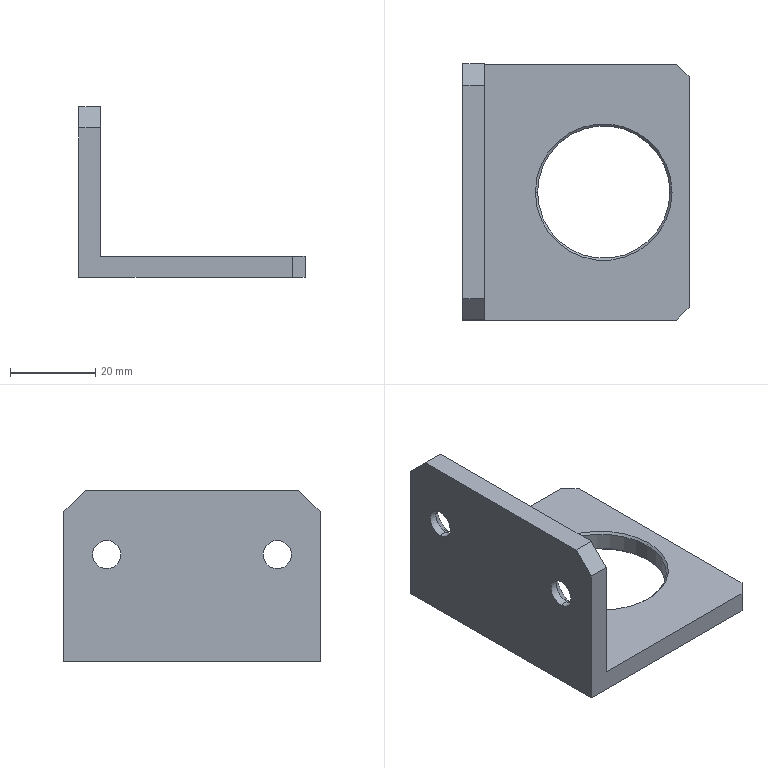Part | SolidWorks | features Chamfer 3, Extrusion 1, HoleWzd 1, ICE 1 | 1 solid | 26 faces | box 53 x 60 x 40 mm | volume 21818 mm3 | plane 12 | cone 8 | cylinder 6 | commonest cylinder face diameters 6.6 x4 31 x2
STEP:
#1=CARTESIAN_POINT('',(17.5,30.,-35.5));
#2=VERTEX_POINT('',#1);
#3=CARTESIAN_POINT('',(48.5,30.,-35.5));
#4=VERTEX_POINT('',#3);
#5=CARTESIAN_POINT('',(33.,30.,-35.5));
#6=DIRECTION('',(0.,0.,1.));
#7=DIRECTION('',(-1.,0.,0.));
#8=AXIS2_PLACEMENT_3D('',#5,#6,#7);
#9=CIRCLE('',#8,15.5);
#10=EDGE_CURVE('',#2,#4,#9,.T.);
#11=ORIENTED_EDGE('',*,*,#10,.F.);
#12=CARTESIAN_POINT('',(17.,30.,-35.));
#13=VERTEX_POINT('',#12);
#14=CARTESIAN_POINT('',(17.,30.,-35.));
#15=DIRECTION('',(-0.7071,0.,0.7071));
#16=VECTOR('',#15,1000.);
#17=LINE('',#14,#16);
#18=EDGE_CURVE('',#2,#13,#17,.T.);
#19=ORIENTED_EDGE('',*,*,#18,.T.);
#20=CARTESIAN_POINT('',(49.,30.,-35.));
#21=VERTEX_POINT('',#20);
#22=CARTESIAN_POINT('',(33.,30.,-35.));
#23=DIRECTION('',(0.,0.,-1.));
#24=DIRECTION('',(-1.,0.,0.));
#25=AXIS2_PLACEMENT_3D('',#22,#23,#24);
#26=CIRCLE('',#25,16.);
#27=EDGE_CURVE('',#21,#13,#26,.T.);
#28=ORIENTED_EDGE('',*,*,#27,.F.);
#29=CARTESIAN_POINT('',(49.,30.,-35.));
#30=DIRECTION('',(0.7071,0.,0.7071));
#31=VECTOR('',#30,1000.);
#32=LINE('',#29,#31);
#33=EDGE_CURVE('',#4,#21,#32,.T.);
#34=ORIENTED_EDGE('',*,*,#33,.F.);
#35=EDGE_LOOP('',(#11,#19,#28,#34));
#36=FACE_OUTER_BOUND('',#35,.T.);
#37=CARTESIAN_POINT('',(33.,30.,-35.));
#38=DIRECTION('',(0.,0.,1.));
#39=DIRECTION('',(1.,0.,0.));
#40=AXIS2_PLACEMENT_3D('',#37,#38,#39);
#41=CONICAL_SURFACE('',#40,16.,0.7854);
#42=ADVANCED_FACE('',(#36),#41,.F.);
#43=CARTESIAN_POINT('',(48.5,30.,-39.5));
#44=VERTEX_POINT('',#43);
#45=CARTESIAN_POINT('',(17.5,30.,-39.5));
#46=VERTEX_POINT('',#45);
#47=CARTESIAN_POINT('',(33.,30.,-39.5));
#48=DIRECTION('',(0.,0.,-1.));
#49=DIRECTION('',(1.,0.,0.));
#50=AXIS2_PLACEMENT_3D('',#47,#48,#49);
#51=CIRCLE('',#50,15.5);
#52=EDGE_CURVE('',#44,#46,#51,.T.);
#53=ORIENTED_EDGE('',*,*,#52,.F.);
#54=CARTESIAN_POINT('',(49.,30.,-40.));
#55=VERTEX_POINT('',#54);
#56=CARTESIAN_POINT('',(48.5,30.,-39.5));
#57=DIRECTION('',(0.7071,0.,-0.7071));
#58=VECTOR('',#57,1000.);
#59=LINE('',#56,#58);
#60=EDGE_CURVE('',#44,#55,#59,.T.);
#61=ORIENTED_EDGE('',*,*,#60,.T.);
#62=CARTESIAN_POINT('',(17.,30.,-40.));
#63=VERTEX_POINT('',#62);
#64=CARTESIAN_POINT('',(33.,30.,-40.));
#65=DIRECTION('',(0.,0.,1.));
#66=DIRECTION('',(1.,0.,0.));
#67=AXIS2_PLACEMENT_3D('',#64,#65,#66);
#68=CIRCLE('',#67,16.);
#69=EDGE_CURVE('',#63,#55,#68,.T.);
#70=ORIENTED_EDGE('',*,*,#69,.F.);
#71=CARTESIAN_POINT('',(17.5,30.,-39.5));
#72=DIRECTION('',(-0.7071,0.,-0.7071));
#73=VECTOR('',#72,1000.);
#74=LINE('',#71,#73);
#75=EDGE_CURVE('',#46,#63,#74,.T.);
#76=ORIENTED_EDGE('',*,*,#75,.F.);
#77=EDGE_LOOP('',(#53,#61,#70,#76));
#78=FACE_OUTER_BOUND('',#77,.T.);
#79=CARTESIAN_POINT('',(33.,30.,-39.5));
#80=DIRECTION('',(0.,0.,-1.));
#81=DIRECTION('',(-1.,0.,0.));
#82=AXIS2_PLACEMENT_3D('',#79,#80,#81);
#83=CONICAL_SURFACE('',#82,15.5,0.7854);
#84=ADVANCED_FACE('',(#78),#83,.F.);
#85=CARTESIAN_POINT('',(1.85,10.,-11.7));
#86=VERTEX_POINT('',#85);
#87=CARTESIAN_POINT('',(1.85,10.,-18.3));
#88=VERTEX_POINT('',#87);
#89=CARTESIAN_POINT('',(1.85,10.,-15.));
#90=DIRECTION('',(1.,0.,0.));
#91=DIRECTION('',(0.,0.,-1.));
#92=AXIS2_PLACEMENT_3D('',#89,#90,#91);
#93=CIRCLE('',#92,3.3);
#94=EDGE_CURVE('',#86,#88,#93,.T.);
#95=ORIENTED_EDGE('',*,*,#94,.F.);
#96=CARTESIAN_POINT('',(5.,10.,-8.55));
#97=VERTEX_POINT('',#96);
#98=CARTESIAN_POINT('',(5.,10.,-8.55));
#99=DIRECTION('',(0.7071,0.,0.7071));
#100=VECTOR('',#99,1000.);
#101=LINE('',#98,#100);
#102=EDGE_CURVE('',#86,#97,#101,.T.);
#103=ORIENTED_EDGE('',*,*,#102,.T.);
#104=CARTESIAN_POINT('',(5.,10.,-21.45));
#105=VERTEX_POINT('',#104);
#106=CARTESIAN_POINT('',(5.,10.,-15.));
#107=DIRECTION('',(1.,0.,0.));
#108=DIRECTION('',(0.,0.,-1.));
#109=AXIS2_PLACEMENT_3D('',#106,#107,#108);
#110=CIRCLE('',#109,6.45);
#111=EDGE_CURVE('',#97,#105,#110,.T.);
#112=ORIENTED_EDGE('',*,*,#111,.T.);
#113=CARTESIAN_POINT('',(5.,10.,-21.45));
#114=DIRECTION('',(0.7071,0.,-0.7071));
#115=VECTOR('',#114,1000.);
#116=LINE('',#113,#115);
#117=EDGE_CURVE('',#88,#105,#116,.T.);
#118=ORIENTED_EDGE('',*,*,#117,.F.);
#119=EDGE_LOOP('',(#95,#103,#112,#118));
#120=FACE_OUTER_BOUND('',#119,.T.);
#121=CARTESIAN_POINT('',(5.,10.,-15.));
#122=DIRECTION('',(1.,0.,0.));
#123=DIRECTION('',(0.,0.,-1.));
#124=AXIS2_PLACEMENT_3D('',#121,#122,#123);
#125=CONICAL_SURFACE('',#124,6.45,0.7854);
#126=ADVANCED_FACE('',(#120),#125,.F.);
#127=CARTESIAN_POINT('',(0.,10.,-11.7));
#128=VERTEX_POINT('',#127);
#129=CARTESIAN_POINT('',(0.,10.,-18.3));
#130=VERTEX_POINT('',#129);
#131=CARTESIAN_POINT('',(0.,10.,-15.));
#132=DIRECTION('',(1.,0.,0.));
#133=DIRECTION('',(0.,0.,-1.));
#134=AXIS2_PLACEMENT_3D('',#131,#132,#133);
#135=CIRCLE('',#134,3.3);
#136=EDGE_CURVE('',#128,#130,#135,.T.);
#137=ORIENTED_EDGE('',*,*,#136,.F.);
#138=CARTESIAN_POINT('',(5.,10.,-11.7));
#139=DIRECTION('',(1.,0.,0.));
#140=VECTOR('',#139,1000.);
#141=LINE('',#138,#140);
#142=EDGE_CURVE('',#128,#86,#141,.T.);
#143=ORIENTED_EDGE('',*,*,#142,.T.);
#144=ORIENTED_EDGE('',*,*,#94,.T.);
#145=CARTESIAN_POINT('',(5.,10.,-18.3));
#146=DIRECTION('',(1.,0.,0.));
#147=VECTOR('',#146,1000.);
#148=LINE('',#145,#147);
#149=EDGE_CURVE('',#130,#88,#148,.T.);
#150=ORIENTED_EDGE('',*,*,#149,.F.);
#151=EDGE_LOOP('',(#137,#143,#144,#150));
#152=FACE_OUTER_BOUND('',#151,.T.);
#153=CARTESIAN_POINT('',(5.,10.,-15.));
#154=DIRECTION('',(1.,0.,0.));
#155=DIRECTION('',(0.,0.,-1.));
#156=AXIS2_PLACEMENT_3D('',#153,#154,#155);
#157=CYLINDRICAL_SURFACE('',#156,3.3);
#158=ADVANCED_FACE('',(#152),#157,.F.);
#159=CARTESIAN_POINT('',(1.85,50.,-11.7));
#160=VERTEX_POINT('',#159);
#161=CARTESIAN_POINT('',(1.85,50.,-18.3));
#162=VERTEX_POINT('',#161);
#163=CARTESIAN_POINT('',(1.85,50.,-15.));
#164=DIRECTION('',(1.,0.,0.));
#165=DIRECTION('',(0.,0.,-1.));
#166=AXIS2_PLACEMENT_3D('',#163,#164,#165);
#167=CIRCLE('',#166,3.3);
#168=EDGE_CURVE('',#160,#162,#167,.T.);
#169=ORIENTED_EDGE('',*,*,#168,.F.);
#170=CARTESIAN_POINT('',(5.,50.,-8.55));
#171=VERTEX_POINT('',#170);
#172=CARTESIAN_POINT('',(5.,50.,-8.55));
#173=DIRECTION('',(0.7071,0.,0.7071));
#174=VECTOR('',#173,1000.);
#175=LINE('',#172,#174);
#176=EDGE_CURVE('',#160,#171,#175,.T.);
#177=ORIENTED_EDGE('',*,*,#176,.T.);
#178=CARTESIAN_POINT('',(5.,50.,-21.45));
#179=VERTEX_POINT('',#178);
#180=CARTESIAN_POINT('',(5.,50.,-15.));
#181=DIRECTION('',(1.,0.,0.));
#182=DIRECTION('',(0.,0.,-1.));
#183=AXIS2_PLACEMENT_3D('',#180,#181,#182);
#184=CIRCLE('',#183,6.45);
#185=EDGE_CURVE('',#171,#179,#184,.T.);
#186=ORIENTED_EDGE('',*,*,#185,.T.);
#187=CARTESIAN_POINT('',(5.,50.,-21.45));
#188=DIRECTION('',(0.7071,0.,-0.7071));
#189=VECTOR('',#188,1000.);
#190=LINE('',#187,#189);
#191=EDGE_CURVE('',#162,#179,#190,.T.);
#192=ORIENTED_EDGE('',*,*,#191,.F.);
#193=EDGE_LOOP('',(#169,#177,#186,#192));
#194=FACE_OUTER_BOUND('',#193,.T.);
#195=CARTESIAN_POINT('',(5.,50.,-15.));
#196=DIRECTION('',(1.,0.,0.));
#197=DIRECTION('',(0.,0.,-1.));
#198=AXIS2_PLACEMENT_3D('',#195,#196,#197);
#199=CONICAL_SURFACE('',#198,6.45,0.7854);
#200=ADVANCED_FACE('',(#194),#199,.F.);
#201=CARTESIAN_POINT('',(0.,50.,-11.7));
#202=VERTEX_POINT('',#201);
#203=CARTESIAN_POINT('',(0.,50.,-18.3));
#204=VERTEX_POINT('',#203);
#205=CARTESIAN_POINT('',(0.,50.,-15.));
#206=DIRECTION('',(1.,0.,0.));
#207=DIRECTION('',(0.,0.,-1.));
#208=AXIS2_PLACEMENT_3D('',#205,#206,#207);
#209=CIRCLE('',#208,3.3);
#210=EDGE_CURVE('',#202,#204,#209,.T.);
#211=ORIENTED_EDGE('',*,*,#210,.F.);
#212=CARTESIAN_POINT('',(5.,50.,-11.7));
#213=DIRECTION('',(1.,0.,0.));
#214=VECTOR('',#213,1000.);
#215=LINE('',#212,#214);
#216=EDGE_CURVE('',#202,#160,#215,.T.);
#217=ORIENTED_EDGE('',*,*,#216,.T.);
#218=ORIENTED_EDGE('',*,*,#168,.T.);
#219=CARTESIAN_POINT('',(5.,50.,-18.3));
#220=DIRECTION('',(1.,0.,0.));
#221=VECTOR('',#220,1000.);
#222=LINE('',#219,#221);
#223=EDGE_CURVE('',#204,#162,#222,.T.);
#224=ORIENTED_EDGE('',*,*,#223,.F.);
#225=EDGE_LOOP('',(#211,#217,#218,#224));
#226=FACE_OUTER_BOUND('',#225,.T.);
#227=CARTESIAN_POINT('',(5.,50.,-15.));
#228=DIRECTION('',(1.,0.,0.));
#229=DIRECTION('',(0.,0.,-1.));
#230=AXIS2_PLACEMENT_3D('',#227,#228,#229);
#231=CYLINDRICAL_SURFACE('',#230,3.3);
#232=ADVANCED_FACE('',(#226),#231,.F.);
#233=ORIENTED_EDGE('',*,*,#10,.T.);
#234=CARTESIAN_POINT('',(48.5,30.,0.));
#235=DIRECTION('',(0.,0.,-1.));
#236=VECTOR('',#235,1000.);
#237=LINE('',#234,#236);
#238=EDGE_CURVE('',#4,#44,#237,.T.);
#239=ORIENTED_EDGE('',*,*,#238,.T.);
#240=ORIENTED_EDGE('',*,*,#52,.T.);
#241=CARTESIAN_POINT('',(17.5,30.,0.));
#242=DIRECTION('',(0.,0.,-1.));
#243=VECTOR('',#242,1000.);
#244=LINE('',#241,#243);
#245=EDGE_CURVE('',#2,#46,#244,.T.);
#246=ORIENTED_EDGE('',*,*,#245,.F.);
#247=EDGE_LOOP('',(#233,#239,#240,#246));
#248=FACE_OUTER_BOUND('',#247,.T.);
#249=CARTESIAN_POINT('',(33.,30.,0.));
#250=DIRECTION('',(0.,0.,-1.));
#251=DIRECTION('',(-1.,0.,0.));
#252=AXIS2_PLACEMENT_3D('',#249,#250,#251);
#253=CYLINDRICAL_SURFACE('',#252,15.5);
#254=ADVANCED_FACE('',(#248),#253,.F.);
#255=CARTESIAN_POINT('',(0.,55.,0.));
#256=VERTEX_POINT('',#255);
#257=CARTESIAN_POINT('',(0.,5.,0.));
#258=VERTEX_POINT('',#257);
#259=CARTESIAN_POINT('',(0.,60.,0.));
#260=DIRECTION('',(0.,-1.,0.));
#261=VECTOR('',#260,1000.);
#262=LINE('',#259,#261);
#263=EDGE_CURVE('',#256,#258,#262,.T.);
#264=ORIENTED_EDGE('',*,*,#263,.T.);
#265=CARTESIAN_POINT('',(5.,5.,0.));
#266=VERTEX_POINT('',#265);
#267=CARTESIAN_POINT('',(5.,5.,0.));
#268=DIRECTION('',(1.,0.,0.));
#269=VECTOR('',#268,1000.);
#270=LINE('',#267,#269);
#271=EDGE_CURVE('',#258,#266,#270,.T.);
#272=ORIENTED_EDGE('',*,*,#271,.T.);
#273=CARTESIAN_POINT('',(5.,55.,0.));
#274=VERTEX_POINT('',#273);
#275=CARTESIAN_POINT('',(5.,60.,0.));
#276=DIRECTION('',(0.,-1.,0.));
#277=VECTOR('',#276,1000.);
#278=LINE('',#275,#277);
#279=EDGE_CURVE('',#274,#266,#278,.T.);
#280=ORIENTED_EDGE('',*,*,#279,.F.);
#281=CARTESIAN_POINT('',(5.,55.,0.));
#282=DIRECTION('',(-1.,0.,0.));
#283=VECTOR('',#282,1000.);
#284=LINE('',#281,#283);
#285=EDGE_CURVE('',#274,#256,#284,.T.);
#286=ORIENTED_EDGE('',*,*,#285,.T.);
#287=EDGE_LOOP('',(#264,#272,#280,#286));
#288=FACE_OUTER_BOUND('',#287,.T.);
#289=CARTESIAN_POINT('',(5.,60.,0.));
#290=DIRECTION('',(0.,0.,-1.));
#291=DIRECTION('',(-1.,0.,0.));
#292=AXIS2_PLACEMENT_3D('',#289,#290,#291);
#293=PLANE('',#292);
#294=ADVANCED_FACE('',(#288),#293,.F.);
#295=CARTESIAN_POINT('',(5.,10.,-15.));
#296=DIRECTION('',(1.,0.,0.));
#297=DIRECTION('',(0.,0.,-1.));
#298=AXIS2_PLACEMENT_3D('',#295,#296,#297);
#299=CIRCLE('',#298,6.45);
#300=EDGE_CURVE('',#105,#97,#299,.T.);
#301=ORIENTED_EDGE('',*,*,#300,.F.);
#302=ORIENTED_EDGE('',*,*,#111,.F.);
#303=EDGE_LOOP('',(#301,#302));
#304=FACE_BOUND('',#303,.T.);
#305=CARTESIAN_POINT('',(5.,50.,-15.));
#306=DIRECTION('',(1.,0.,0.));
#307=DIRECTION('',(0.,0.,-1.));
#308=AXIS2_PLACEMENT_3D('',#305,#306,#307);
#309=CIRCLE('',#308,6.45);
#310=EDGE_CURVE('',#179,#171,#309,.T.);
#311=ORIENTED_EDGE('',*,*,#310,.F.);
#312=ORIENTED_EDGE('',*,*,#185,.F.);
#313=EDGE_LOOP('',(#311,#312));
#314=FACE_BOUND('',#313,.T.);
#315=ORIENTED_EDGE('',*,*,#279,.T.);
#316=CARTESIAN_POINT('',(5.,0.,-5.));
#317=VERTEX_POINT('',#316);
#318=CARTESIAN_POINT('',(5.,5.,0.));
#319=DIRECTION('',(0.,-0.7071,-0.7071));
#320=VECTOR('',#319,1000.);
#321=LINE('',#318,#320);
#322=EDGE_CURVE('',#266,#317,#321,.T.);
#323=ORIENTED_EDGE('',*,*,#322,.T.);
#324=CARTESIAN_POINT('',(5.,0.,-35.));
#325=VERTEX_POINT('',#324);
#326=CARTESIAN_POINT('',(5.,0.,0.));
#327=DIRECTION('',(0.,0.,-1.));
#328=VECTOR('',#327,1000.);
#329=LINE('',#326,#328);
#330=EDGE_CURVE('',#317,#325,#329,.T.);
#331=ORIENTED_EDGE('',*,*,#330,.T.);
#332=CARTESIAN_POINT('',(5.,60.,-35.));
#333=VERTEX_POINT('',#332);
#334=CARTESIAN_POINT('',(5.,60.,-35.));
#335=DIRECTION('',(0.,-1.,0.));
#336=VECTOR('',#335,1000.);
#337=LINE('',#334,#336);
#338=EDGE_CURVE('',#333,#325,#337,.T.);
#339=ORIENTED_EDGE('',*,*,#338,.F.);
#340=CARTESIAN_POINT('',(5.,60.,-5.));
#341=VERTEX_POINT('',#340);
#342=CARTESIAN_POINT('',(5.,60.,0.));
#343=DIRECTION('',(0.,0.,-1.));
#344=VECTOR('',#343,1000.);
#345=LINE('',#342,#344);
#346=EDGE_CURVE('',#341,#333,#345,.T.);
#347=ORIENTED_EDGE('',*,*,#346,.F.);
#348=CARTESIAN_POINT('',(5.,60.,-5.));
#349=DIRECTION('',(0.,-0.7071,0.7071));
#350=VECTOR('',#349,1000.);
#351=LINE('',#348,#350);
#352=EDGE_CURVE('',#341,#274,#351,.T.);
#353=ORIENTED_EDGE('',*,*,#352,.T.);
#354=EDGE_LOOP('',(#315,#323,#331,#339,#347,#353));
#355=FACE_OUTER_BOUND('',#354,.T.);
#356=CARTESIAN_POINT('',(5.,60.,0.));
#357=DIRECTION('',(-1.,0.,0.));
#358=DIRECTION('',(0.,0.,1.));
#359=AXIS2_PLACEMENT_3D('',#356,#357,#358);
#360=PLANE('',#359);
#361=ADVANCED_FACE('',(#304,#314,#355),#360,.F.);
#362=ORIENTED_EDGE('',*,*,#27,.T.);
#363=CARTESIAN_POINT('',(33.,30.,-35.));
#364=DIRECTION('',(0.,0.,-1.));
#365=DIRECTION('',(-1.,0.,0.));
#366=AXIS2_PLACEMENT_3D('',#363,#364,#365);
#367=CIRCLE('',#366,16.);
#368=EDGE_CURVE('',#13,#21,#367,.T.);
#369=ORIENTED_EDGE('',*,*,#368,.T.);
#370=EDGE_LOOP('',(#362,#369));
#371=FACE_BOUND('',#370,.T.);
#372=CARTESIAN_POINT('',(53.,57.,-35.));
#373=VERTEX_POINT('',#372);
#374=CARTESIAN_POINT('',(53.,3.,-35.));
#375=VERTEX_POINT('',#374);
#376=CARTESIAN_POINT('',(53.,60.,-35.));
#377=DIRECTION('',(0.,-1.,0.));
#378=VECTOR('',#377,1000.);
#379=LINE('',#376,#378);
#380=EDGE_CURVE('',#373,#375,#379,.T.);
#381=ORIENTED_EDGE('',*,*,#380,.F.);
#382=CARTESIAN_POINT('',(50.,60.,-35.));
#383=VERTEX_POINT('',#382);
#384=CARTESIAN_POINT('',(50.,60.,-35.));
#385=DIRECTION('',(-0.7071,0.7071,0.));
#386=VECTOR('',#385,1000.);
#387=LINE('',#384,#386);
#388=EDGE_CURVE('',#373,#383,#387,.T.);
#389=ORIENTED_EDGE('',*,*,#388,.T.);
#390=CARTESIAN_POINT('',(5.,60.,-35.));
#391=DIRECTION('',(1.,0.,0.));
#392=VECTOR('',#391,1000.);
#393=LINE('',#390,#392);
#394=EDGE_CURVE('',#333,#383,#393,.T.);
#395=ORIENTED_EDGE('',*,*,#394,.F.);
#396=ORIENTED_EDGE('',*,*,#338,.T.);
#397=CARTESIAN_POINT('',(50.,0.,-35.));
#398=VERTEX_POINT('',#397);
#399=CARTESIAN_POINT('',(5.,0.,-35.));
#400=DIRECTION('',(1.,0.,0.));
#401=VECTOR('',#400,1000.);
#402=LINE('',#399,#401);
#403=EDGE_CURVE('',#325,#398,#402,.T.);
#404=ORIENTED_EDGE('',*,*,#403,.T.);
#405=CARTESIAN_POINT('',(53.,3.,-35.));
#406=DIRECTION('',(0.7071,0.7071,0.));
#407=VECTOR('',#406,1000.);
#408=LINE('',#405,#407);
#409=EDGE_CURVE('',#398,#375,#408,.T.);
#410=ORIENTED_EDGE('',*,*,#409,.T.);
#411=EDGE_LOOP('',(#381,#389,#395,#396,#404,#410));
#412=FACE_OUTER_BOUND('',#411,.T.);
#413=CARTESIAN_POINT('',(5.,60.,-35.));
#414=DIRECTION('',(0.,0.,-1.));
#415=DIRECTION('',(-1.,0.,0.));
#416=AXIS2_PLACEMENT_3D('',#413,#414,#415);
#417=PLANE('',#416);
#418=ADVANCED_FACE('',(#371,#412),#417,.F.);
#419=CARTESIAN_POINT('',(53.,57.,-40.));
#420=VERTEX_POINT('',#419);
#421=CARTESIAN_POINT('',(53.,3.,-40.));
#422=VERTEX_POINT('',#421);
#423=CARTESIAN_POINT('',(53.,60.,-40.));
#424=DIRECTION('',(0.,-1.,0.));
#425=VECTOR('',#424,1000.);
#426=LINE('',#423,#425);
#427=EDGE_CURVE('',#420,#422,#426,.T.);
#428=ORIENTED_EDGE('',*,*,#427,.F.);
#429=CARTESIAN_POINT('',(53.,57.,-40.));
#430=DIRECTION('',(0.,0.,1.));
#431=VECTOR('',#430,1000.);
#432=LINE('',#429,#431);
#433=EDGE_CURVE('',#420,#373,#432,.T.);
#434=ORIENTED_EDGE('',*,*,#433,.T.);
#435=ORIENTED_EDGE('',*,*,#380,.T.);
#436=CARTESIAN_POINT('',(53.,3.,-40.));
#437=DIRECTION('',(0.,0.,-1.));
#438=VECTOR('',#437,1000.);
#439=LINE('',#436,#438);
#440=EDGE_CURVE('',#375,#422,#439,.T.);
#441=ORIENTED_EDGE('',*,*,#440,.T.);
#442=EDGE_LOOP('',(#428,#434,#435,#441));
#443=FACE_OUTER_BOUND('',#442,.T.);
#444=CARTESIAN_POINT('',(53.,60.,-40.));
#445=DIRECTION('',(-1.,0.,0.));
#446=DIRECTION('',(0.,0.,1.));
#447=AXIS2_PLACEMENT_3D('',#444,#445,#446);
#448=PLANE('',#447);
#449=ADVANCED_FACE('',(#443),#448,.F.);
#450=ORIENTED_EDGE('',*,*,#69,.T.);
#451=CARTESIAN_POINT('',(33.,30.,-40.));
#452=DIRECTION('',(0.,0.,1.));
#453=DIRECTION('',(1.,0.,0.));
#454=AXIS2_PLACEMENT_3D('',#451,#452,#453);
#455=CIRCLE('',#454,16.);
#456=EDGE_CURVE('',#55,#63,#455,.T.);
#457=ORIENTED_EDGE('',*,*,#456,.T.);
#458=EDGE_LOOP('',(#450,#457));
#459=FACE_BOUND('',#458,.T.);
#460=CARTESIAN_POINT('',(50.,60.,-40.));
#461=VERTEX_POINT('',#460);
#462=CARTESIAN_POINT('',(0.,60.,-40.));
#463=VERTEX_POINT('',#462);
#464=CARTESIAN_POINT('',(0.,60.,-40.));
#465=DIRECTION('',(-1.,0.,0.));
#466=VECTOR('',#465,1000.);
#467=LINE('',#464,#466);
#468=EDGE_CURVE('',#461,#463,#467,.T.);
#469=ORIENTED_EDGE('',*,*,#468,.F.);
#470=CARTESIAN_POINT('',(50.,60.,-40.));
#471=DIRECTION('',(0.7071,-0.7071,0.));
#472=VECTOR('',#471,1000.);
#473=LINE('',#470,#472);
#474=EDGE_CURVE('',#461,#420,#473,.T.);
#475=ORIENTED_EDGE('',*,*,#474,.T.);
#476=ORIENTED_EDGE('',*,*,#427,.T.);
#477=CARTESIAN_POINT('',(50.,0.,-40.));
#478=VERTEX_POINT('',#477);
#479=CARTESIAN_POINT('',(53.,3.,-40.));
#480=DIRECTION('',(-0.7071,-0.7071,0.));
#481=VECTOR('',#480,1000.);
#482=LINE('',#479,#481);
#483=EDGE_CURVE('',#422,#478,#482,.T.);
#484=ORIENTED_EDGE('',*,*,#483,.T.);
#485=CARTESIAN_POINT('',(0.,0.,-40.));
#486=VERTEX_POINT('',#485);
#487=CARTESIAN_POINT('',(0.,0.,-40.));
#488=DIRECTION('',(-1.,0.,0.));
#489=VECTOR('',#488,1000.);
#490=LINE('',#487,#489);
#491=EDGE_CURVE('',#478,#486,#490,.T.);
#492=ORIENTED_EDGE('',*,*,#491,.T.);
#493=CARTESIAN_POINT('',(0.,60.,-40.));
#494=DIRECTION('',(0.,-1.,0.));
#495=VECTOR('',#494,1000.);
#496=LINE('',#493,#495);
#497=EDGE_CURVE('',#463,#486,#496,.T.);
#498=ORIENTED_EDGE('',*,*,#497,.F.);
#499=EDGE_LOOP('',(#469,#475,#476,#484,#492,#498));
#500=FACE_OUTER_BOUND('',#499,.T.);
#501=CARTESIAN_POINT('',(0.,60.,-40.));
#502=DIRECTION('',(0.,0.,1.));
#503=DIRECTION('',(1.,0.,0.));
#504=AXIS2_PLACEMENT_3D('',#501,#502,#503);
#505=PLANE('',#504);
#506=ADVANCED_FACE('',(#459,#500),#505,.F.);
#507=CARTESIAN_POINT('',(0.,10.,-15.));
#508=DIRECTION('',(1.,0.,0.));
#509=DIRECTION('',(0.,0.,-1.));
#510=AXIS2_PLACEMENT_3D('',#507,#508,#509);
#511=CIRCLE('',#510,3.3);
#512=EDGE_CURVE('',#130,#128,#511,.T.);
#513=ORIENTED_EDGE('',*,*,#512,.T.);
#514=ORIENTED_EDGE('',*,*,#136,.T.);
#515=EDGE_LOOP('',(#513,#514));
#516=FACE_BOUND('',#515,.T.);
#517=CARTESIAN_POINT('',(0.,50.,-15.));
#518=DIRECTION('',(1.,0.,0.));
#519=DIRECTION('',(0.,0.,-1.));
#520=AXIS2_PLACEMENT_3D('',#517,#518,#519);
#521=CIRCLE('',#520,3.3);
#522=EDGE_CURVE('',#204,#202,#521,.T.);
#523=ORIENTED_EDGE('',*,*,#522,.T.);
#524=ORIENTED_EDGE('',*,*,#210,.T.);
#525=EDGE_LOOP('',(#523,#524));
#526=FACE_BOUND('',#525,.T.);
#527=CARTESIAN_POINT('',(0.,0.,-5.));
#528=VERTEX_POINT('',#527);
#529=CARTESIAN_POINT('',(0.,0.,0.));
#530=DIRECTION('',(0.,0.,1.));
#531=VECTOR('',#530,1000.);
#532=LINE('',#529,#531);
#533=EDGE_CURVE('',#486,#528,#532,.T.);
#534=ORIENTED_EDGE('',*,*,#533,.T.);
#535=CARTESIAN_POINT('',(0.,5.,0.));
#536=DIRECTION('',(0.,0.7071,0.7071));
#537=VECTOR('',#536,1000.);
#538=LINE('',#535,#537);
#539=EDGE_CURVE('',#528,#258,#538,.T.);
#540=ORIENTED_EDGE('',*,*,#539,.T.);
#541=ORIENTED_EDGE('',*,*,#263,.F.);
#542=CARTESIAN_POINT('',(0.,60.,-5.));
#543=VERTEX_POINT('',#542);
#544=CARTESIAN_POINT('',(0.,60.,-5.));
#545=DIRECTION('',(0.,0.7071,-0.7071));
#546=VECTOR('',#545,1000.);
#547=LINE('',#544,#546);
#548=EDGE_CURVE('',#256,#543,#547,.T.);
#549=ORIENTED_EDGE('',*,*,#548,.T.);
#550=CARTESIAN_POINT('',(0.,60.,0.));
#551=DIRECTION('',(0.,0.,1.));
#552=VECTOR('',#551,1000.);
#553=LINE('',#550,#552);
#554=EDGE_CURVE('',#463,#543,#553,.T.);
#555=ORIENTED_EDGE('',*,*,#554,.F.);
#556=ORIENTED_EDGE('',*,*,#497,.T.);
#557=EDGE_LOOP('',(#534,#540,#541,#549,#555,#556));
#558=FACE_OUTER_BOUND('',#557,.T.);
#559=CARTESIAN_POINT('',(0.,60.,0.));
#560=DIRECTION('',(1.,0.,0.));
#561=DIRECTION('',(0.,0.,-1.));
#562=AXIS2_PLACEMENT_3D('',#559,#560,#561);
#563=PLANE('',#562);
#564=ADVANCED_FACE('',(#516,#526,#558),#563,.F.);
#565=ORIENTED_EDGE('',*,*,#554,.T.);
#566=CARTESIAN_POINT('',(0.,60.,-5.));
#567=DIRECTION('',(1.,0.,0.));
#568=VECTOR('',#567,1000.);
#569=LINE('',#566,#568);
#570=EDGE_CURVE('',#543,#341,#569,.T.);
#571=ORIENTED_EDGE('',*,*,#570,.T.);
#572=ORIENTED_EDGE('',*,*,#346,.T.);
#573=ORIENTED_EDGE('',*,*,#394,.T.);
#574=CARTESIAN_POINT('',(50.,60.,0.));
#575=DIRECTION('',(0.,0.,-1.));
#576=VECTOR('',#575,1000.);
#577=LINE('',#574,#576);
#578=EDGE_CURVE('',#383,#461,#577,.T.);
#579=ORIENTED_EDGE('',*,*,#578,.T.);
#580=ORIENTED_EDGE('',*,*,#468,.T.);
#581=EDGE_LOOP('',(#565,#571,#572,#573,#579,#580));
#582=FACE_OUTER_BOUND('',#581,.T.);
#583=CARTESIAN_POINT('',(0.,60.,0.));
#584=DIRECTION('',(0.,-1.,0.));
#585=DIRECTION('',(0.,0.,-1.));
#586=AXIS2_PLACEMENT_3D('',#583,#584,#585);
#587=PLANE('',#586);
#588=ADVANCED_FACE('',(#582),#587,.F.);
#589=ORIENTED_EDGE('',*,*,#330,.F.);
#590=CARTESIAN_POINT('',(0.,0.,-5.));
#591=DIRECTION('',(-1.,0.,0.));
#592=VECTOR('',#591,1000.);
#593=LINE('',#590,#592);
#594=EDGE_CURVE('',#317,#528,#593,.T.);
#595=ORIENTED_EDGE('',*,*,#594,.T.);
#596=ORIENTED_EDGE('',*,*,#533,.F.);
#597=ORIENTED_EDGE('',*,*,#491,.F.);
#598=CARTESIAN_POINT('',(50.,0.,-35.));
#599=DIRECTION('',(0.,0.,1.));
#600=VECTOR('',#599,1000.);
#601=LINE('',#598,#600);
#602=EDGE_CURVE('',#478,#398,#601,.T.);
#603=ORIENTED_EDGE('',*,*,#602,.T.);
#604=ORIENTED_EDGE('',*,*,#403,.F.);
#605=EDGE_LOOP('',(#589,#595,#596,#597,#603,#604));
#606=FACE_OUTER_BOUND('',#605,.T.);
#607=CARTESIAN_POINT('',(0.,0.,0.));
#608=DIRECTION('',(0.,-1.,0.));
#609=DIRECTION('',(0.,0.,-1.));
#610=AXIS2_PLACEMENT_3D('',#607,#608,#609);
#611=PLANE('',#610);
#612=ADVANCED_FACE('',(#606),#611,.T.);
#613=ORIENTED_EDGE('',*,*,#238,.F.);
#614=CARTESIAN_POINT('',(33.,30.,-35.5));
#615=DIRECTION('',(0.,0.,1.));
#616=DIRECTION('',(-1.,0.,0.));
#617=AXIS2_PLACEMENT_3D('',#614,#615,#616);
#618=CIRCLE('',#617,15.5);
#619=EDGE_CURVE('',#4,#2,#618,.T.);
#620=ORIENTED_EDGE('',*,*,#619,.T.);
#621=ORIENTED_EDGE('',*,*,#245,.T.);
#622=CARTESIAN_POINT('',(33.,30.,-39.5));
#623=DIRECTION('',(0.,0.,-1.));
#624=DIRECTION('',(1.,0.,0.));
#625=AXIS2_PLACEMENT_3D('',#622,#623,#624);
#626=CIRCLE('',#625,15.5);
#627=EDGE_CURVE('',#46,#44,#626,.T.);
#628=ORIENTED_EDGE('',*,*,#627,.T.);
#629=EDGE_LOOP('',(#613,#620,#621,#628));
#630=FACE_OUTER_BOUND('',#629,.T.);
#631=CARTESIAN_POINT('',(33.,30.,0.));
#632=DIRECTION('',(0.,0.,-1.));
#633=DIRECTION('',(-1.,0.,0.));
#634=AXIS2_PLACEMENT_3D('',#631,#632,#633);
#635=CYLINDRICAL_SURFACE('',#634,15.5);
#636=ADVANCED_FACE('',(#630),#635,.F.);
#637=ORIENTED_EDGE('',*,*,#388,.F.);
#638=ORIENTED_EDGE('',*,*,#433,.F.);
#639=ORIENTED_EDGE('',*,*,#474,.F.);
#640=ORIENTED_EDGE('',*,*,#578,.F.);
#641=EDGE_LOOP('',(#637,#638,#639,#640));
#642=FACE_OUTER_BOUND('',#641,.T.);
#643=CARTESIAN_POINT('',(50.,60.,0.));
#644=DIRECTION('',(-0.7071,-0.7071,0.));
#645=DIRECTION('',(0.7071,-0.7071,0.));
#646=AXIS2_PLACEMENT_3D('',#643,#644,#645);
#647=PLANE('',#646);
#648=ADVANCED_FACE('',(#642),#647,.F.);
#649=ORIENTED_EDGE('',*,*,#409,.F.);
#650=ORIENTED_EDGE('',*,*,#602,.F.);
#651=ORIENTED_EDGE('',*,*,#483,.F.);
#652=ORIENTED_EDGE('',*,*,#440,.F.);
#653=EDGE_LOOP('',(#649,#650,#651,#652));
#654=FACE_OUTER_BOUND('',#653,.T.);
#655=CARTESIAN_POINT('',(53.,3.,-40.));
#656=DIRECTION('',(0.7071,-0.7071,0.));
#657=DIRECTION('',(0.7071,0.7071,0.));
#658=AXIS2_PLACEMENT_3D('',#655,#656,#657);
#659=PLANE('',#658);
#660=ADVANCED_FACE('',(#654),#659,.T.);
#661=ORIENTED_EDGE('',*,*,#539,.F.);
#662=ORIENTED_EDGE('',*,*,#594,.F.);
#663=ORIENTED_EDGE('',*,*,#322,.F.);
#664=ORIENTED_EDGE('',*,*,#271,.F.);
#665=EDGE_LOOP('',(#661,#662,#663,#664));
#666=FACE_OUTER_BOUND('',#665,.T.);
#667=CARTESIAN_POINT('',(5.,5.,0.));
#668=DIRECTION('',(0.,-0.7071,0.7071));
#669=DIRECTION('',(0.,-0.7071,-0.7071));
#670=AXIS2_PLACEMENT_3D('',#667,#668,#669);
#671=PLANE('',#670);
#672=ADVANCED_FACE('',(#666),#671,.T.);
#673=ORIENTED_EDGE('',*,*,#548,.F.);
#674=ORIENTED_EDGE('',*,*,#285,.F.);
#675=ORIENTED_EDGE('',*,*,#352,.F.);
#676=ORIENTED_EDGE('',*,*,#570,.F.);
#677=EDGE_LOOP('',(#673,#674,#675,#676));
#678=FACE_OUTER_BOUND('',#677,.T.);
#679=CARTESIAN_POINT('',(0.,60.,-5.));
#680=DIRECTION('',(0.,-0.7071,-0.7071));
#681=DIRECTION('',(0.,0.7071,-0.7071));
#682=AXIS2_PLACEMENT_3D('',#679,#680,#681);
#683=PLANE('',#682);
#684=ADVANCED_FACE('',(#678),#683,.F.);
#685=ORIENTED_EDGE('',*,*,#216,.F.);
#686=ORIENTED_EDGE('',*,*,#522,.F.);
#687=ORIENTED_EDGE('',*,*,#223,.T.);
#688=CARTESIAN_POINT('',(1.85,50.,-15.));
#689=DIRECTION('',(1.,0.,0.));
#690=DIRECTION('',(0.,0.,-1.));
#691=AXIS2_PLACEMENT_3D('',#688,#689,#690);
#692=CIRCLE('',#691,3.3);
#693=EDGE_CURVE('',#162,#160,#692,.T.);
#694=ORIENTED_EDGE('',*,*,#693,.T.);
#695=EDGE_LOOP('',(#685,#686,#687,#694));
#696=FACE_OUTER_BOUND('',#695,.T.);
#697=CARTESIAN_POINT('',(5.,50.,-15.));
#698=DIRECTION('',(1.,0.,0.));
#699=DIRECTION('',(0.,0.,-1.));
#700=AXIS2_PLACEMENT_3D('',#697,#698,#699);
#701=CYLINDRICAL_SURFACE('',#700,3.3);
#702=ADVANCED_FACE('',(#696),#701,.F.);
#703=ORIENTED_EDGE('',*,*,#176,.F.);
#704=ORIENTED_EDGE('',*,*,#693,.F.);
#705=ORIENTED_EDGE('',*,*,#191,.T.);
#706=ORIENTED_EDGE('',*,*,#310,.T.);
#707=EDGE_LOOP('',(#703,#704,#705,#706));
#708=FACE_OUTER_BOUND('',#707,.T.);
#709=CARTESIAN_POINT('',(5.,50.,-15.));
#710=DIRECTION('',(1.,0.,0.));
#711=DIRECTION('',(0.,0.,-1.));
#712=AXIS2_PLACEMENT_3D('',#709,#710,#711);
#713=CONICAL_SURFACE('',#712,6.45,0.7854);
#714=ADVANCED_FACE('',(#708),#713,.F.);
#715=ORIENTED_EDGE('',*,*,#142,.F.);
#716=ORIENTED_EDGE('',*,*,#512,.F.);
#717=ORIENTED_EDGE('',*,*,#149,.T.);
#718=CARTESIAN_POINT('',(1.85,10.,-15.));
#719=DIRECTION('',(1.,0.,0.));
#720=DIRECTION('',(0.,0.,-1.));
#721=AXIS2_PLACEMENT_3D('',#718,#719,#720);
#722=CIRCLE('',#721,3.3);
#723=EDGE_CURVE('',#88,#86,#722,.T.);
#724=ORIENTED_EDGE('',*,*,#723,.T.);
#725=EDGE_LOOP('',(#715,#716,#717,#724));
#726=FACE_OUTER_BOUND('',#725,.T.);
#727=CARTESIAN_POINT('',(5.,10.,-15.));
#728=DIRECTION('',(1.,0.,0.));
#729=DIRECTION('',(0.,0.,-1.));
#730=AXIS2_PLACEMENT_3D('',#727,#728,#729);
#731=CYLINDRICAL_SURFACE('',#730,3.3);
#732=ADVANCED_FACE('',(#726),#731,.F.);
#733=ORIENTED_EDGE('',*,*,#102,.F.);
#734=ORIENTED_EDGE('',*,*,#723,.F.);
#735=ORIENTED_EDGE('',*,*,#117,.T.);
#736=ORIENTED_EDGE('',*,*,#300,.T.);
#737=EDGE_LOOP('',(#733,#734,#735,#736));
#738=FACE_OUTER_BOUND('',#737,.T.);
#739=CARTESIAN_POINT('',(5.,10.,-15.));
#740=DIRECTION('',(1.,0.,0.));
#741=DIRECTION('',(0.,0.,-1.));
#742=AXIS2_PLACEMENT_3D('',#739,#740,#741);
#743=CONICAL_SURFACE('',#742,6.45,0.7854);
#744=ADVANCED_FACE('',(#738),#743,.F.);
#745=ORIENTED_EDGE('',*,*,#60,.F.);
#746=ORIENTED_EDGE('',*,*,#627,.F.);
#747=ORIENTED_EDGE('',*,*,#75,.T.);
#748=ORIENTED_EDGE('',*,*,#456,.F.);
#749=EDGE_LOOP('',(#745,#746,#747,#748));
#750=FACE_OUTER_BOUND('',#749,.T.);
#751=CARTESIAN_POINT('',(33.,30.,-39.5));
#752=DIRECTION('',(0.,0.,-1.));
#753=DIRECTION('',(-1.,0.,0.));
#754=AXIS2_PLACEMENT_3D('',#751,#752,#753);
#755=CONICAL_SURFACE('',#754,15.5,0.7854);
#756=ADVANCED_FACE('',(#750),#755,.F.);
#757=ORIENTED_EDGE('',*,*,#18,.F.);
#758=ORIENTED_EDGE('',*,*,#619,.F.);
#759=ORIENTED_EDGE('',*,*,#33,.T.);
#760=ORIENTED_EDGE('',*,*,#368,.F.);
#761=EDGE_LOOP('',(#757,#758,#759,#760));
#762=FACE_OUTER_BOUND('',#761,.T.);
#763=CARTESIAN_POINT('',(33.,30.,-35.));
#764=DIRECTION('',(0.,0.,1.));
#765=DIRECTION('',(1.,0.,0.));
#766=AXIS2_PLACEMENT_3D('',#763,#764,#765);
#767=CONICAL_SURFACE('',#766,16.,0.7854);
#768=ADVANCED_FACE('',(#762),#767,.F.);
#769=CLOSED_SHELL('',(#42,#84,#126,#158,#200,#232,#254,#294,#361,#418,#449,#506,#564,#588,#612,#636,#648,#660,#672,#684,#702,#714,#732,#744,#756,#768));
#770=MANIFOLD_SOLID_BREP('',#769);
#771=CARTESIAN_POINT('',(0.,0.,0.));
#772=DIRECTION('',(0.,0.,1.));
#773=DIRECTION('',(1.,0.,0.));
#774=AXIS2_PLACEMENT_3D('',#771,#772,#773);
#775=(LENGTH_UNIT()NAMED_UNIT(*)SI_UNIT(.MILLI.,.METRE.));
#776=UNCERTAINTY_MEASURE_WITH_UNIT(LENGTH_MEASURE(0.00001),#775,'','');
#777=(NAMED_UNIT(*)PLANE_ANGLE_UNIT()SI_UNIT($,.RADIAN.));
#778=(NAMED_UNIT(*)SI_UNIT($,.STERADIAN.)SOLID_ANGLE_UNIT());
#779=(GEOMETRIC_REPRESENTATION_CONTEXT(3)GLOBAL_UNCERTAINTY_ASSIGNED_CONTEXT((#776))GLOBAL_UNIT_ASSIGNED_CONTEXT((#775,#777,#778))REPRESENTATION_CONTEXT('',''));
#780=ADVANCED_BREP_SHAPE_REPRESENTATION('',(#770,#774),#779);